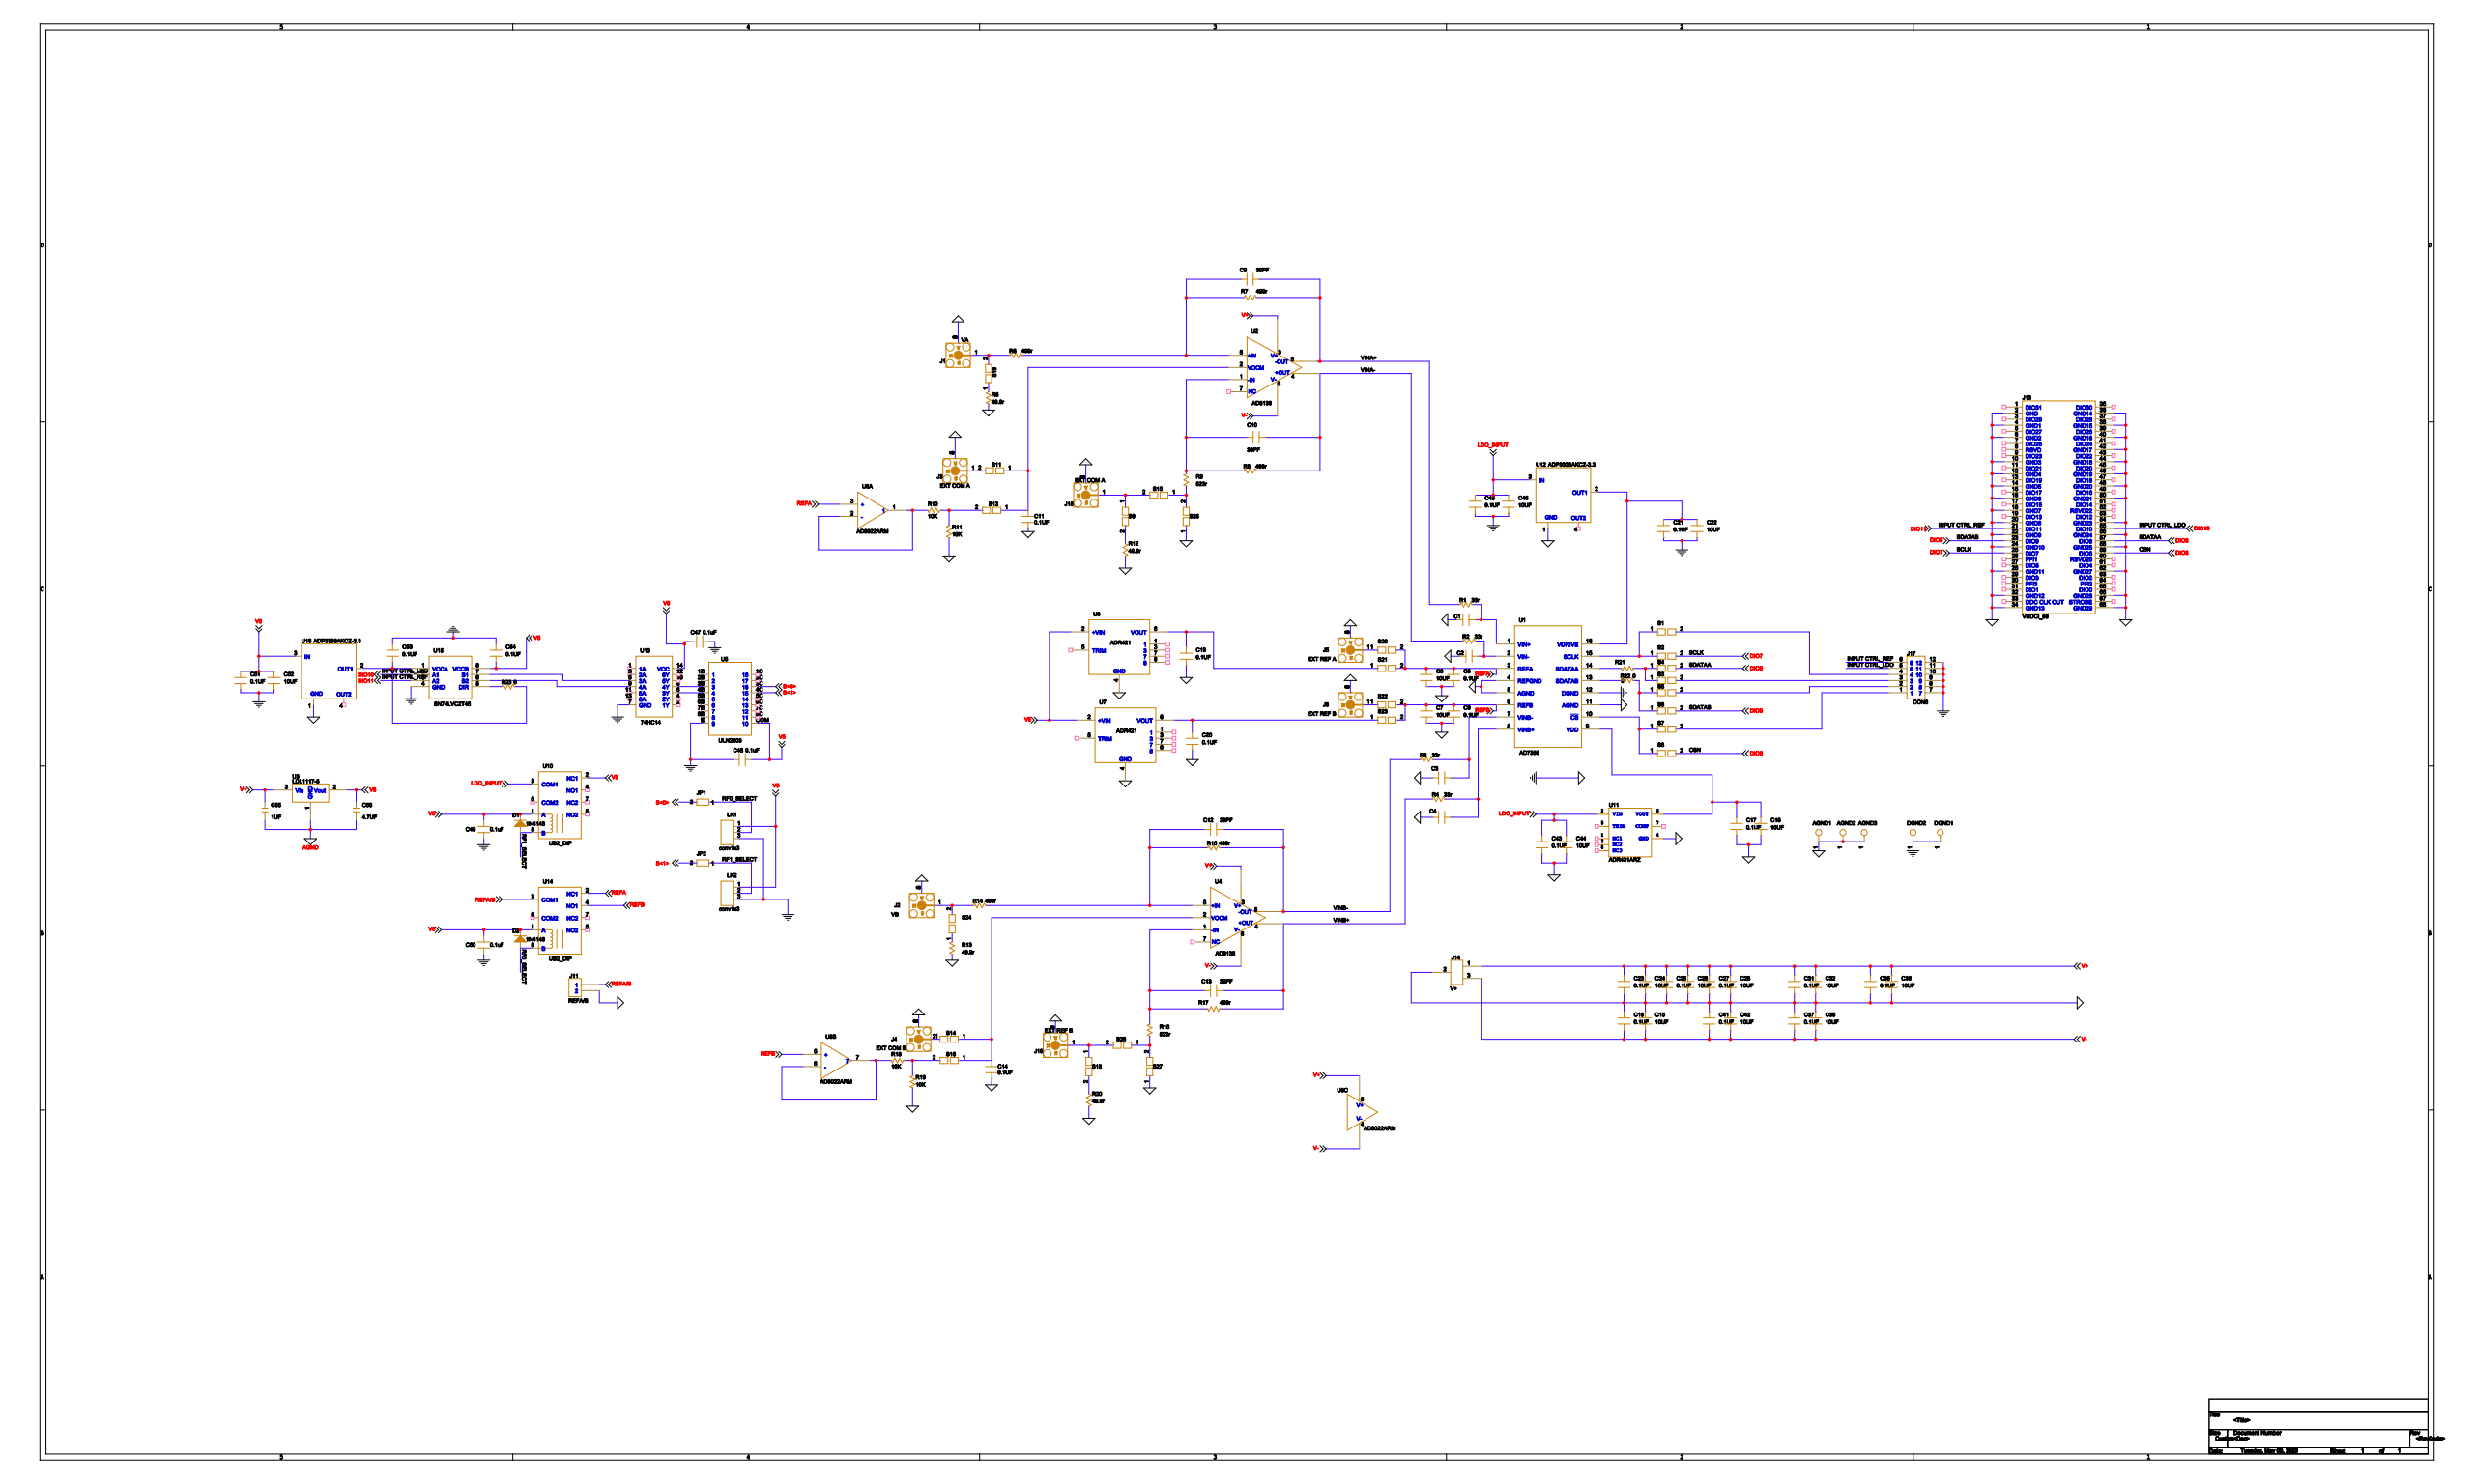Circuit board | Cadence Allegro | 135 parts | 71 nets
Bill of materials:
SYM_NAME,COMP_DEVICE_TYPE,COMP_VALUE,COMP_TOL,COMP_CLASS,REFDES
TPC50D30,TESTPOINT_TPC50D30_AGND1,AGND1,,IC,AGND1
TPC50D30,TESTPOINT_TPC50D30_AGND2,AGND2,,IC,AGND2
TPC50D30,TESTPOINT_TPC50D30_AGND3,AGND3,,IC,AGND3
R0603,C_R0603_C,C,,IC,C1
R0603,C_R0603_C,C,,IC,C2
R0603,C_R0603_C,C,,IC,C3
R0603,C_R0603_C,C,,IC,C4
R0603,C_R0603_0.1UF,0.1UF,,IC,C5
1206_C,C_1206_C_10UF,10UF,,IC,C6
1206_C,C_1206_C_10UF,10UF,,IC,C7
R0603,C_R0603_0.1UF,0.1UF,,IC,C8
R0603,C_R0603_39PF,39PF,,IC,C9
R0603,C_R0603_39PF,39PF,,IC,C10
R0603,C_R0603_0.1UF,0.1UF,,IC,C11
R0603,C_R0603_39PF,39PF,,IC,C12
R0603,C_R0603_39PF,39PF,,IC,C13
R0603,C_R0603_0.1UF,0.1UF,,IC,C14
1206_C,C_1206_C_10UF,10UF,,IC,C15
R0603,C_R0603_0.1UF,0.1UF,,IC,C16
0402,C_0402_0.1UF,0.1UF,,IC,C17
1206_C,C_1206_C_10UF,10UF,,IC,C18
R0603,C_R0603_0.1UF,0.1UF,,IC,C19
R0603,C_R0603_0.1UF,0.1UF,,IC,C20
0402,C_0402_0.1UF,0.1UF,,IC,C21
1206_C,C_1206_C_10UF,10UF,,IC,C22
R0603,C_R0603_0.1UF,0.1UF,,IC,C23
1206_C,C_1206_C_10UF,10UF,,IC,C24
R0603,C_R0603_0.1UF,0.1UF,,IC,C25
1206_C,C_1206_C_10UF,10UF,,IC,C26
R0603,C_R0603_0.1UF,0.1UF,,IC,C27
1206_C,C_1206_C_10UF,10UF,,IC,C28
R0603,C_R0603_0.1UF,0.1UF,,IC,C31
1206_C,C_1206_C_10UF,10UF,,IC,C32
R0603,C_R0603_0.1UF,0.1UF,,IC,C35
1206_C,C_1206_C_10UF,10UF,,IC,C36
R0603,C_R0603_0.1UF,0.1UF,,IC,C37
1206_C,C_1206_C_10UF,10UF,,IC,C38
R0603,C_R0603_0.1UF,0.1UF,,IC,C41
1206_C,C_1206_C_10UF,10UF,,IC,C42
0402,C_0402_0.1UF,0.1UF,,IC,C43
1206_C,C_1206_C_10UF,10UF,,IC,C44
0402,C_0402_0.1UF,0.1UF,,IC,C45
1206_C,C_1206_C_10UF,10UF,,IC,C46
C0603,CAP_C0603_0.1UF,0.1uF,,IC,C47
C0603,CAP_C0603_0.1UF,0.1uF,,IC,C48
C0603,CAP_C0603_0.1UF,0.1uF,,IC,C49
C0603,CAP_C0603_0.1UF,0.1uF,,IC,C50
0402,C_0402_0.1UF,0.1UF,,IC,C51
1206_C,C_1206_C_10UF,10UF,,IC,C52
0402,C_0402_0.1UF,0.1UF,,IC,C53
0402,C_0402_0.1UF,0.1UF,,IC,C54
C0402,CAPNP_V_0_C0402_1UF,1UF,,IC,C55
C0402,CAPNP_V_0_C0402_4.7UF,4.7UF,,IC,C56
SOD_123,1N4148_SOD_123_1N4148,1N4148,,IC,D1
SOD_123,1N4148_SOD_123_1N4148,1N4148,,IC,D2
TPC50D30,TESTPOINT_TPC50D30_DGND1,DGND1,,IC,DGND1
TPC50D30,TESTPOINT_TPC50D30_DGND2,DGND2,,IC,DGND2
SMB_V-RJ45,SMA_SMB_V-RJ45_VA,VA,,IC,J1
SMB_V-RJ45,SMA_SMB_V-RJ45_VB,VB,,IC,J2
SMB_V-RJ45,SMA_SMB_V-RJ45_EXT COM A,EXT COM A,,IC,J3
SMB_V-RJ45,SMA_SMB_V-RJ45_EXT COM B,EXT COM B,,IC,J4
SMB_V-RJ45,SMA_SMB_V-RJ45_EXT REF A,EXT REF A,,IC,J5
SMB_V-RJ45,SMA_SMB_V-RJ45_EXT REF B,EXT REF B,,IC,J6
POW2_BOLT,CON2_POW2_BOLT_REFA/B,REFA/B,,IC,J11
VHDCI_68,VHDCI_68_U7_1_VHDCI_68_VHDCI_68,VHDCI_68,,IC,J13
POW3_BOLT,CON3_POW3_BOLT_V+,V+,,IC,J14
SMB_V-RJ45,SMA_SMB_V-RJ45_EXT COM A,EXT COM A,,IC,J15
CON6X2,CON6X2_CON6X2_CON6,CON6,,IC,J17
SMB_V-RJ45,SMA_SMB_V-RJ45_EXT REF B,EXT REF B,,IC,J18
HDR_1X2,CON2/_HDR_1X2_CON2/,con2/,,IC,JP1
HDR_1X2,CON2/_HDR_1X2_CON2/,con2/,,IC,JP2
HDR254M-1X3,CONV_HDR254M-1X3_CONV1X3,conv1x3,,IC,LK1
HDR254M-1X3,CONV_HDR254M-1X3_CONV1X3,conv1x3,,IC,LK2
R0603,R_R0603_33R,33r,,IC,R1
R0603,R_R0603_33R,33r,,IC,R2
R0603,R_R0603_33R,33r,,IC,R3
R0603,R_R0603_33R,33r,,IC,R4
R0603,R_R0603_49.9R,49.9r,,IC,R5
R0603,R_R0603_499R,499r,,IC,R6
R0603,R_R0603_499R,499r,,IC,R7
R0603,R_R0603_499R,499r,,IC,R8
R0603,R_R0603_523R,523r,,IC,R9
R0603,R_R0603_10K,10K,,IC,R10
R0603,R_R0603_10K,10K,,IC,R11
R0603,R_R0603_49.9R,49.9r,,IC,R12
R0603,R_R0603_49.9R,49.9r,,IC,R13
R0603,R_R0603_499R,499r,,IC,R14
R0603,R_R0603_499R,499r,,IC,R15
R0603,R_R0603_523R,523r,,IC,R16
R0603,R_R0603_499R,499r,,IC,R17
R0603,R_R0603_10K,10K,,IC,R18
R0603,R_R0603_10K,10K,,IC,R19
R0603,R_R0603_49.9R,49.9r,,IC,R20
R0603,R_R0603_0,0,,IC,R21
R0603,R_R0603_0,0,,IC,R22
R0603,R_R0603_0,0,,IC,R23
R0603,S_R0603_S,S,,IC,S1
R0603,S_R0603_S,S,,IC,S2
R0603,S_R0603_S,S,,IC,S3
R0603,S_R0603_S,S,,IC,S4
R0603,S_R0603_S,S,,IC,S5
R0603,S_R0603_S,S,,IC,S6
R0603,S_R0603_S,S,,IC,S7
R0603,S_R0603_S,S,,IC,S8
R0603,S_R0603_S,S,,IC,S9
R0603,S_R0603_S,S,,IC,S11
R0603,S_R0603_S,S,,IC,S13
R0603,S_R0603_S,S,,IC,S14
R0603,S_R0603_S,S,,IC,S15
R0603,S_R0603_S,S,,IC,S16
R0603,S_R0603_S,S,,IC,S18
R0603,S_R0603_S,S,,IC,S19
R0603,S_R0603_S,S,,IC,S20
R0603,S_R0603_S,S,,IC,S21
R0603,S_R0603_S,S,,IC,S22
R0603,S_R0603_S,S,,IC,S23
R0603,S_R0603_S,S,,IC,S24
R0603,S_R0603_S,S,,IC,S25
R0603,S_R0603_S,S,,IC,S26
R0603,S_R0603_S,S,,IC,S27
AD7356CHAZUO,AD7356_0_AD7356CHAZUO_AD7356,AD7356,,IC,U1
SOIC8_TB,AD8138_0_SOIC8_TB_AD8138,AD8138,,IC,U2
SOT-223,AMS1117-3.3_SOT-223_LDL1117-5,LDL1117-5,,IC,U3
SOIC8_TB,AD8138_0_SOIC8_TB_AD8138,AD8138,,IC,U4
ULN2803,ULN2803_0_ULN2803_ULN2803,ULN2803,,IC,U5
SOIC8_TB,ADR421_0_SOIC8_TB_ADR421,ADR421,,IC,U6
SOIC8_TB,ADR421_0_SOIC8_TB_ADR421,ADR421,,IC,U7
MSOP_8,AD8022ARM_MSOP_8_AD8022ARM,AD8022ARM,,IC,U8
UB2_DIP,UB2_DIP_UB2_DIP_UB2_DIP,UB2_DIP,,IC,U10
SOIC-8,ADR431ARZ_U4_0_SOIC-8_ADR431ARZ,ADR431ARZ,,IC,U11
SOT223-2,ADP3338AKCZ-3.3_SOT223-2_ADP333,ADP3338AKCZ-3.3,,IC,U12
74HC14,74HC14_74HC14_74HC14,74HC14,,IC,U13
UB2_DIP,UB2_DIP_UB2_DIP_UB2_DIP,UB2_DIP,,IC,U14
SOP8_DCT,SN74LVC2T45_SOP8_DCT_SN74LVC2T4,SN74LVC2T45,,IC,U15
SOT223-2,ADP3338AKCZ-3.3_SOT223-2_ADP333,ADP3338AKCZ-3.3,,IC,U16
Netlist (net: part-pin ...):
N14942432: J17-1 S7-2
AGND: AGND1-1 AGND2-1 AGND3-1 C1-2 C2-2 C3-2 C4-2 C5-1 C6-2 C7-2 C8-1 C11-2 C14-2 C15-1 C16-1 C17-2 C18-2 C19-1 C20-2 C21-2 C22-2 C23-2 C24-2 C25-2 C26-2 C27-2 C28-2 C31-2 C32-2 C35-2 C36-2 C37-1 C38-1 C41-1 C42-1 C43-2 C44-2 C45-2 C46-2 C51-2 C52-2 C55-2 C56-2 DGND1-1 DGND2-1 J1-2 J1-3 J1-4 J1-5 J2-2 J2-3 J2-4 J2-5 J3-2 J3-3 J3-4 J3-5 J4-2 J4-3 J4-4 J4-5 J5-2 J5-3 J5-4 J5-5 J6-2 J6-3 J6-4 J6-5 J11-2 J13-2 J13-4 J13-6 J13-10 J13-12 J13-14 J13-16 J13-18 J13-20 J13-22 J13-24 J13-28 J13-32 J13-34 J13-36 J13-38 J13-40 J13-42 J13-44 J13-46 J13-48 J13-50 J13-54 J13-56 J13-58 J13-62 J13-66 J13-68 J14-2 J15-2 J15-3 J15-4 J15-5 J17-7 J17-8 J17-9 J17-10 J17-11 J17-12 J18-2 J18-3 J18-4 J18-5 R5-1 R11-1 R12-2 R13-1 R19-1 R20-2 S25-1 S27-1 U1-4 U1-5 U1-11 U1-12 U3-1 U6-4 U7-4 U11-4 U12-1 U16-1
N14942389: J17-2 S5-2
N14942212: J17-3 S3-2
N14942143: J17-4 S1-2
DIO10: J13-55 J17-5 U15-2
DIO11: J13-21 J17-6 U15-3
N14920247: U13-5 U15-7
N14920361: U13-9 U15-6
N14939775: R23-1 U15-5
GND: C47-1 C48-2 C49-1 C50-1 C53-1 C54-1 LK1-3 LK2-3 U5-E U13-7 U15-4
N14938014: C53-2 R23-2 U15-1 U16-2
V5: C47-2 C48-1 C49-2 C50-2 C51-1 C52-1 C54-2 C56-1 D1-1 D2-1 LK1-1 LK2-1 U3-2 U5-COM U6-2 U7-2 U10-1 U10-2 U13-14 U14-1 U15-8 U16-3
V+: C23-1 C24-1 C25-1 C26-1 C27-1 C28-1 C31-1 C32-1 C35-1 C36-1 C55-1 J14-1 U2-3 U3-3 U4-3 U8-8
REFA/B: J11-1 U14-3
RF1_SELECT: D1-2 JP2-1 LK2-2 U10-8
RF0_SELECT: D2-2 JP1-1 LK1-2 U14-8
S<0>: JP1-2 U5-3C
S<1>: JP2-2 U5-4C
LDO_INPUT: C43-1 C44-1 C45-1 C46-1 U10-3 U11-2 U12-3
REFA: C5-2 C6-1 S20-2 S21-2 U1-3 U8-3 U14-2
REFB: C7-1 C8-2 S22-2 S23-2 U1-6 U8-5 U14-4
N262498: C17-1 C18-1 U1-9 U11-6
N260062: C21-1 C22-1 U1-16 U12-2
N14920385: U5-4B U13-6
N14920369: U5-3B U13-8
DIO6: J13-59 S8-2
DIO7: J13-25 S2-2
DIO8: J13-57 S4-2
DIO9: J13-23 S6-2
N262410: S7-1 S8-1 U1-10
N261604: S1-1 S2-1 U1-15
N261768: R21-2 U1-14
N261850: R22-1 U1-13
N260750: C1-1 R1-2 U1-1
N261316: C2-1 R2-2 U1-2
N262490: C4-1 R4-2 U1-8
N262402: C3-1 R3-2 U1-7
N259692: C10-1 R8-1 R9-2 U2-1
VINA-: C10-2 R2-1 R8-2 U2-4
VINB-: C12-1 R3-1 R15-2 U4-5
N262898: C12-2 R14-2 R15-1 U4-8
N263204: C13-1 R16-2 R17-2 U4-1
VINB+: C13-2 R4-1 R17-1 U4-4
VINA+: C9-1 R1-1 R7-2 U2-5
N259438: C9-2 R6-2 R7-1 U2-8
N259670: C11-1 S11-1 S13-1 U2-2
N263182: C14-1 S14-1 S16-1 U4-2
V-: C15-2 C16-2 C37-2 C38-2 C41-2 C42-2 J14-3 U2-6 U4-6 U8-4
N261182: C19-2 S21-1 U6-6
N262386: C20-1 S23-1 U7-6
N259624: J1-1 R6-1 S19-2
N259970: J15-1 S9-1 S15-2
N259838: J3-1 S11-2
N264154: J18-1 S18-1 S26-2
N262262: J6-1 S22-1
N263140: J2-1 R14-1 S24-2
N264090: J4-1 S14-2
N261498: J5-1 S20-1
N260154: R10-1 R11-2 S13-2
N260142: R10-2 U8-1 U8-2
N264236: R18-1 R19-2 S16-2
N264224: R18-2 U8-6 U8-7
N260262: R12-1 S9-2
N263200: R13-2 S24-1
N264340: R20-1 S18-2
N259700: R5-2 S19-1
N264012: R16-1 S26-1 S27-2
N259940: R9-1 S15-1 S25-2
N261772: R21-1 S3-1 S4-1
N261854: R22-2 S5-1 S6-1